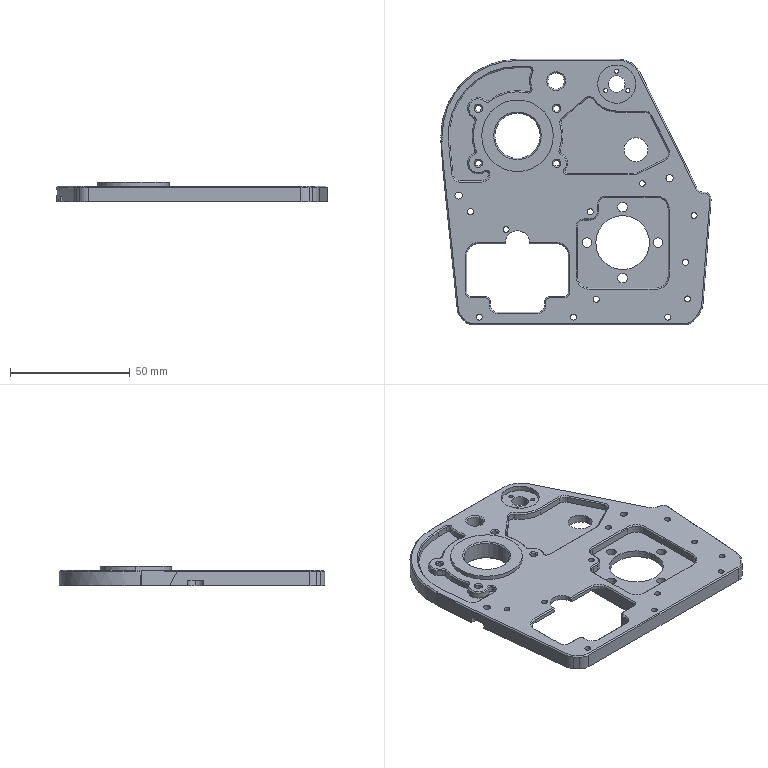Part | NX | features BREP 1 | 1 solid | 289 faces | box 113.061 x 111.064 x 8.2 mm | volume 45327 mm3 | cylinder 133 | plane 81 | cone 75 | commonest cylinder face diameters 2.5 x30 4 x15 2 x14 6 x14 10 x13 1.7 x6